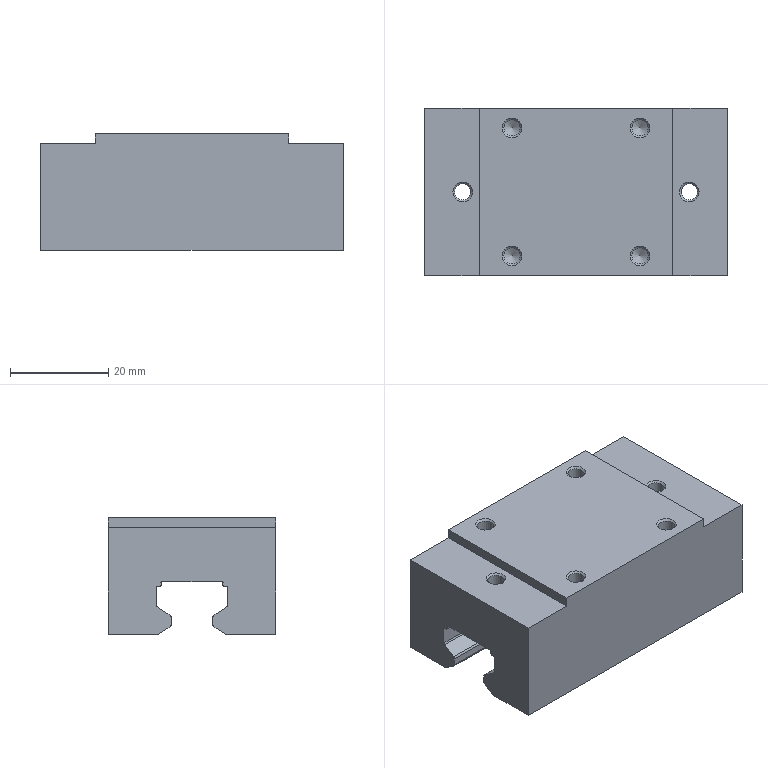Part | STEP file | Tube feed_id846_x_t | 1 solid | 52 faces | box 61.4 x 34 x 23.7 mm | volume 39681 mm3 | plane 20 | cylinder 20 | cone 12 | commonest cylinder face diameters 1 x7 0.6 x6 3.3 x6 1.005 x1